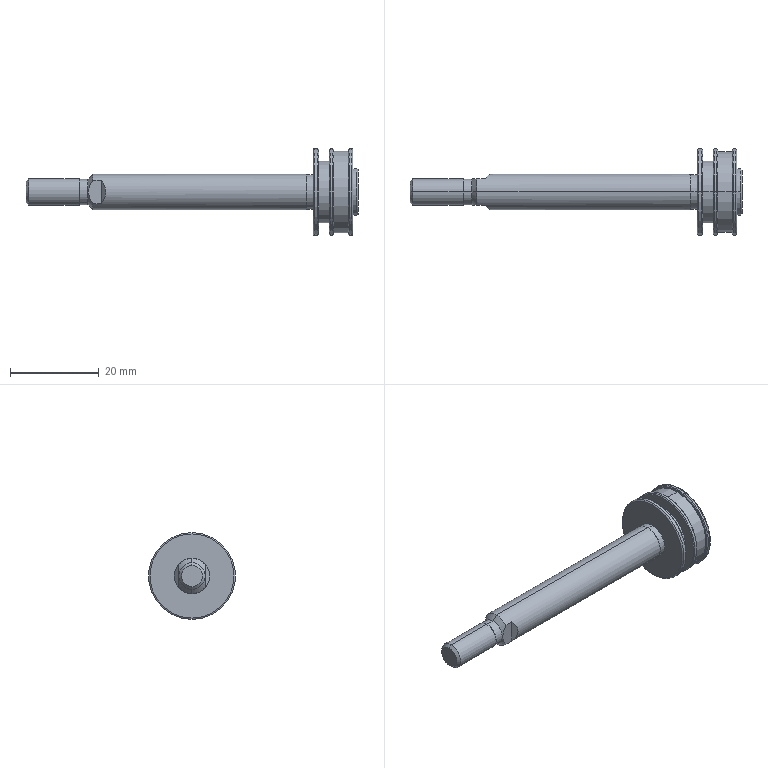Part | STEP file | 1 solid | 52 faces | box 75 x 19.6 x 19.6 mm | volume 5220 mm3 | cylinder 20 | cone 14 | plane 14 | torus 4 | commonest cylinder face diameters 19.6 x6 5.8 x2 6 x2 7.8 x2 8 x2 10.6 x2